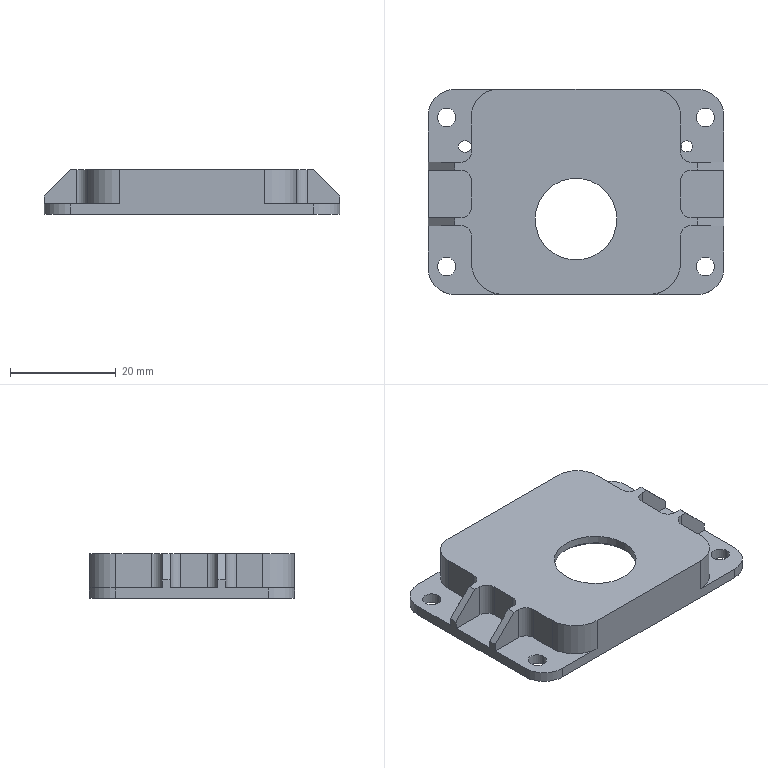NC program | NX | posted with a generic post | part box 56 x 38.85 x 8.5 mm
Lines 291 to 2522 of 3190, first 1751 of 2228 lines:
(CAVITY_MILL_COPY_COPY , TOOL : D4)
N556 T11 M6
N558 G54
N560 G17 G0 G90 X-11.864 Y14.625 S9500 M3
N562 G43 Z30. H11
N564 Z0.6
N566 G94 G1 Z-0.4 F1000.
N568 X-12.037 Y14.925
N570 G3 X-12.903 Y15.425 R1.
N572 G1 X-14.7 F1400.
N574 G3 X-15.8 Y14.325 R1.1
N576 G1 Y12.528
N578 G3 X-15.3 Y11.662 R1.
N580 G1 X-15. Y11.489
N582 Z0.6
N584 G0 Z30.
N586 X-11.764 Y14.525
N588 Z0.2
N590 G1 Z-0.8 F1000.
N592 X-11.937 Y14.825
N594 G3 X-12.803 Y15.325 R1.
N596 G1 X-14.7 F1400.
N598 G3 X-15.7 Y14.325 R1.
N600 G1 Y12.428
N602 G3 X-15.2 Y11.562 R1.
N604 G1 X-14.9 Y11.389
N606 Z0.2
N608 G0 X-11.764 Y14.525 Z-0.2
N610 G1 Z-1.2 F1000.
N612 X-11.937 Y14.825
N614 G3 X-12.803 Y15.325 R1.
N616 G1 X-14.7 F1400.
N618 G3 X-15.7 Y14.325 R1.
N620 G1 Y12.428
N622 G3 X-15.2 Y11.562 R1.
N624 G1 X-14.9 Y11.389
N626 Z-0.2
N628 G0 X-11.764 Y14.525 Z-0.6
N630 G1 Z-1.6 F1000.
N632 X-11.937 Y14.825
N634 G3 X-12.803 Y15.325 R1.
N636 G1 X-14.7 F1400.
N638 G3 X-15.7 Y14.325 R1.
N640 G1 Y12.428
N642 G3 X-15.2 Y11.562 R1.
N644 G1 X-14.9 Y11.389
N646 Z-0.6
N648 G0 X-11.764 Y14.525 Z-1.
N650 G1 Z-2. F1000.
N652 X-11.937 Y14.825
N654 G3 X-12.803 Y15.325 R1.
N656 G1 X-14.7 F1400.
N658 G3 X-15.7 Y14.325 R1.
N660 G1 Y12.428
N662 G3 X-15.2 Y11.562 R1.
N664 G1 X-14.9 Y11.389
N666 Z-1.
N668 G0 X-11.764 Y14.525 Z-1.375
N670 G1 Z-2.375 F1000.
N672 X-11.937 Y14.825
N674 G3 X-12.803 Y15.325 R1.
N676 G1 X-14.7 F1400.
N678 G3 X-15.7 Y14.325 R1.
N680 G1 Y12.428
N682 G3 X-15.2 Y11.562 R1.
N684 G1 X-14.9 Y11.389
N686 Z-1.375
N688 G0 X-11.764 Y14.525 Z-1.75
N690 G1 Z-2.75 F1000.
N692 X-11.937 Y14.825
N694 G3 X-12.803 Y15.325 R1.
N696 G1 X-14.7 F1400.
N698 G3 X-15.7 Y14.325 R1.
N700 G1 Y12.428
N702 G3 X-15.2 Y11.562 R1.
N704 G1 X-14.9 Y11.389
N706 Z-1.75
N708 G0 X-11.764 Y14.525 Z-2.125
N710 G1 Z-3.125 F1000.
N712 X-11.937 Y14.825
N714 G3 X-12.803 Y15.325 R1.
N716 G1 X-14.7 F1400.
N718 G3 X-15.7 Y14.325 R1.
N720 G1 Y12.428
N722 G3 X-15.2 Y11.562 R1.
N724 G1 X-14.9 Y11.389
N726 Z-2.125
N728 G0 X-11.764 Y14.525 Z-2.5
N730 G1 Z-3.5 F1000.
N732 X-11.937 Y14.825
N734 G3 X-12.803 Y15.325 R1.
N736 G1 X-14.7 F1400.
N738 G3 X-15.7 Y14.325 R1.
N740 G1 Y12.428
N742 G3 X-15.2 Y11.562 R1.
N744 G1 X-14.9 Y11.389
N746 Z-2.5
N748 G0 X-6.729 Y4.936 Z-2.875
N750 G1 Z-3.875 F1000.
N752 X-7.565 Y4.93
N754 G3 X-8.427 Y4.423 R1.
N756 G1 X-13.24 Y7.152
N758 G2 X-13.3 Y7.825 R3.8 F1400.
N760 G1 Y13.525
N762 X-13.9
N764 Y7.152
N766 X-13.24
N768 X-11.468 Y7.471
N770 G2 X-11.5 Y7.825 R2.
N772 G1 Y15.325
N774 X-14.7
N776 G3 X-15.7 Y14.325 R1.
N778 G1 Y5.352
N780 X-11.2
N782 G2 X-9.2 Y3.352 R2.
N784 G1 Y3.145
N786 G3 X-8.728 Y3.565 R0.5
N788 G2 X-7.411 Y5.416 R2.56
N790 G3 X-7.17 Y6.005 R0.5
N792 G2 X-8. Y5.825 R2.
N794 G1 X-9.5
N796 G2 X-11.468 Y7.471 R2.
N798 G3 X-11.579 Y7.705 R0.5
N800 G1 Z-2.875
N802 G0 X-6.729 Y4.936 Z-3.25
N804 G1 Z-4.25 F1000.
N806 X-7.565 Y4.93
N808 G3 X-8.427 Y4.423 R1.
N810 G1 X-13.24 Y7.152
N812 G2 X-13.3 Y7.825 R3.8 F1400.
N814 G1 Y13.525
N816 X-13.9
N818 Y7.152
N820 X-13.24
N822 X-11.468 Y7.471
N824 G2 X-11.5 Y7.825 R2.
N826 G1 Y15.325
N828 X-14.7
N830 G3 X-15.7 Y14.325 R1.
N832 G1 Y5.352
N834 X-11.2
N836 G2 X-9.2 Y3.352 R2.
N838 G1 Y3.145
N840 G3 X-8.728 Y3.565 R0.5
N842 G2 X-7.411 Y5.416 R2.56
N844 G3 X-7.17 Y6.005 R0.5
N846 G2 X-8. Y5.825 R2.
N848 G1 X-9.5
N850 G2 X-11.468 Y7.471 R2.
N852 G3 X-11.579 Y7.705 R0.5
N854 G1 Z-3.25
N856 G0 Z30.
N858 X-6.729 Y4.936
N860 Z-3.625
N862 G1 Z-4.625 F1000.
N864 X-7.565 Y4.93
N866 G3 X-8.427 Y4.423 R1.
N868 G1 X-13.24 Y7.152
N870 G2 X-13.3 Y7.825 R3.8 F1400.
N872 G1 Y13.525
N874 X-13.9
N876 Y7.152
N878 X-13.24
N880 X-11.468 Y7.471
N882 G2 X-11.5 Y7.825 R2.
N884 G1 Y15.325
N886 X-14.7
N888 G3 X-15.7 Y14.325 R1.
N890 G1 Y5.352
N892 X-11.2
N894 G2 X-9.2 Y3.352 R2.
N896 G1 Y3.145
N898 G3 X-8.728 Y3.565 R0.5
N900 G2 X-7.411 Y5.416 R2.56
N902 G3 X-7.17 Y6.005 R0.5
N904 G2 X-8. Y5.825 R2.
N906 G1 X-9.5
N908 G2 X-11.468 Y7.471 R2.
N910 G3 X-11.579 Y7.705 R0.5
N912 G1 Z-3.625
N914 G0 Z30.
N916 X-6.729 Y4.936
N918 Z-4.
N920 G1 Z-5. F1000.
N922 X-7.565 Y4.93
N924 G3 X-8.427 Y4.423 R1.
N926 G1 X-13.24 Y7.152
N928 G2 X-13.3 Y7.825 R3.8 F1400.
N930 G1 Y13.525
N932 X-13.9
N934 Y7.152
N936 X-13.24
N938 X-11.468 Y7.471
N940 G2 X-11.5 Y7.825 R2.
N942 G1 Y15.325
N944 X-14.7
N946 G3 X-15.7 Y14.325 R1.
N948 G1 Y5.352
N950 X-11.2
N952 G2 X-9.2 Y3.352 R2.
N954 G1 Y3.145
N956 G3 X-8.728 Y3.565 R0.5
N958 G2 X-7.411 Y5.416 R2.56
N960 G3 X-7.17 Y6.005 R0.5
N962 G2 X-8. Y5.825 R2.
N964 G1 X-9.5
N966 G2 X-11.468 Y7.471 R2.
N968 G3 X-11.579 Y7.705 R0.5
N970 G1 Z-4.
N972 G0 Z30.
N974 X-6.729 Y4.936
N976 Z-4.375
N978 G1 Z-5.375 F1000.
N980 X-7.565 Y4.93
N982 G3 X-8.427 Y4.423 R1.
N984 G1 X-13.24 Y7.152
N986 G2 X-13.3 Y7.825 R3.8 F1400.
N988 G1 Y13.525
N990 X-13.9
N992 Y7.152
N994 X-13.24
N996 X-11.468 Y7.471
N998 G2 X-11.5 Y7.825 R2.
N1000 G1 Y15.325
N1002 X-14.7
N1004 G3 X-15.7 Y14.325 R1.
N1006 G1 Y5.352
N1008 X-11.2
N1010 G2 X-9.2 Y3.352 R2.
N1012 G1 Y3.145
N1014 G3 X-8.728 Y3.565 R0.5
N1016 G2 X-7.411 Y5.416 R2.56
N1018 G3 X-7.17 Y6.005 R0.5
N1020 G2 X-8. Y5.825 R2.
N1022 G1 X-9.5
N1024 G2 X-11.468 Y7.471 R2.
N1026 G3 X-11.579 Y7.705 R0.5
N1028 G1 Z-4.375
N1030 G0 Z30.
N1032 X-6.729 Y4.936
N1034 Z-4.75
N1036 G1 Z-5.75 F1000.
N1038 X-7.565 Y4.93
N1040 G3 X-8.427 Y4.423 R1.
N1042 G1 X-13.24 Y7.152
N1044 G2 X-13.3 Y7.825 R3.8 F1400.
N1046 G1 Y13.525
N1048 X-13.9
N1050 Y7.152
N1052 X-13.24
N1054 X-11.468 Y7.471
N1056 G2 X-11.5 Y7.825 R2.
N1058 G1 Y15.325
N1060 X-14.7
N1062 G3 X-15.7 Y14.325 R1.
N1064 G1 Y5.352
N1066 X-11.2
N1068 G2 X-9.2 Y3.352 R2.
N1070 G1 Y3.145
N1072 G3 X-8.728 Y3.565 R0.5
N1074 G2 X-7.411 Y5.416 R2.56
N1076 G3 X-7.17 Y6.005 R0.5
N1078 G2 X-8. Y5.825 R2.
N1080 G1 X-9.5
N1082 G2 X-11.468 Y7.471 R2.
N1084 G3 X-11.579 Y7.705 R0.5
N1086 G1 Z-4.75
N1088 G0 Z30.
N1090 X-6.729 Y4.936
N1092 Z-5.125
N1094 G1 Z-6.125 F1000.
N1096 X-7.565 Y4.93
N1098 G3 X-8.427 Y4.423 R1.
N1100 G1 X-13.24 Y7.152
N1102 G2 X-13.3 Y7.825 R3.8 F1400.
N1104 G1 Y13.525
N1106 X-13.9
N1108 Y7.152
N1110 X-13.24
N1112 X-11.468 Y7.471
N1114 G2 X-11.5 Y7.825 R2.
N1116 G1 Y15.325
N1118 X-14.7
N1120 G3 X-15.7 Y14.325 R1.
N1122 G1 Y5.352
N1124 X-11.2
N1126 G2 X-9.2 Y3.352 R2.
N1128 G1 Y3.145
N1130 G3 X-8.728 Y3.565 R0.5
N1132 G2 X-7.411 Y5.416 R2.56
N1134 G3 X-7.17 Y6.005 R0.5
N1136 G2 X-8. Y5.825 R2.
N1138 G1 X-9.5
N1140 G2 X-11.468 Y7.471 R2.
N1142 G3 X-11.579 Y7.705 R0.5
N1144 G1 Z-5.125
N1146 G0 Z30.
N1148 X-6.729 Y4.936
N1150 Z-5.5
N1152 G1 Z-6.5 F1000.
N1154 X-7.565 Y4.93
N1156 G3 X-8.427 Y4.423 R1.
N1158 G1 X-13.24 Y7.152
N1160 G2 X-13.3 Y7.825 R3.8 F1400.
N1162 G1 Y13.525
N1164 X-13.9
N1166 Y7.152
N1168 X-13.24
N1170 X-11.468 Y7.471
N1172 G2 X-11.5 Y7.825 R2.
N1174 G1 Y15.325
N1176 X-14.7
N1178 G3 X-15.7 Y14.325 R1.
N1180 G1 Y5.352
N1182 X-11.2
N1184 G2 X-9.2 Y3.352 R2.
N1186 G1 Y3.145
N1188 G3 X-8.728 Y3.565 R0.5
N1190 G2 X-7.411 Y5.416 R2.56
N1192 G3 X-7.17 Y6.005 R0.5
N1194 G2 X-8. Y5.825 R2.
N1196 G1 X-9.5
N1198 G2 X-11.468 Y7.471 R2.
N1200 G3 X-11.579 Y7.705 R0.5
N1202 G1 Z-5.5
N1204 G0 Z30.
N1206 X-1.859 Y5.254
N1208 Z-2.875
N1210 G1 Z-3.875 F1000.
N1212 X-1.824 Y5.407
N1214 G3 X-2.115 Y6.363 R1.
N1216 G2 X-2.75 Y7.825 R2. F1400.
N1218 G1 Y15.325
N1220 X-6.
N1222 Y7.825
N1224 G2 X-6.635 Y6.363 R2.
N1226 G3 X-6.926 Y5.407 R1.
N1228 G1 X-6.891 Y5.254
N1230 Z-2.875
N1232 G0 X-1.859 Z-3.25
N1234 G1 Z-4.25 F1000.
N1236 X-1.824 Y5.407
N1238 G3 X-2.115 Y6.363 R1.
N1240 G2 X-2.75 Y7.825 R2. F1400.
N1242 G1 Y15.325
N1244 X-6.
N1246 Y7.825
N1248 G2 X-6.635 Y6.363 R2.
N1250 G3 X-6.926 Y5.407 R1.
N1252 G1 X-6.891 Y5.254
N1254 Z-3.25
N1256 G0 X-1.859 Z-3.625
N1258 G1 Z-4.625 F1000.
N1260 X-1.824 Y5.407
N1262 G3 X-2.115 Y6.363 R1.
N1264 G2 X-2.75 Y7.825 R2. F1400.
N1266 G1 Y15.325
N1268 X-6.
N1270 Y7.825
N1272 G2 X-6.635 Y6.363 R2.
N1274 G3 X-6.926 Y5.407 R1.
N1276 G1 X-6.891 Y5.254
N1278 Z-3.625
N1280 G0 X-1.859 Z-4.
N1282 G1 Z-5. F1000.
N1284 X-1.824 Y5.407
N1286 G3 X-2.115 Y6.363 R1.
N1288 G2 X-2.75 Y7.825 R2. F1400.
N1290 G1 Y15.325
N1292 X-6.
N1294 Y7.825
N1296 G2 X-6.635 Y6.363 R2.
N1298 G3 X-6.926 Y5.407 R1.
N1300 G1 X-6.891 Y5.254
N1302 Z-4.
N1304 G0 X-1.859 Z-4.375
N1306 G1 Z-5.375 F1000.
N1308 X-1.824 Y5.407
N1310 G3 X-2.115 Y6.363 R1.
N1312 G2 X-2.75 Y7.825 R2. F1400.
N1314 G1 Y15.325
N1316 X-6.
N1318 Y7.825
N1320 G2 X-6.635 Y6.363 R2.
N1322 G3 X-6.926 Y5.407 R1.
N1324 G1 X-6.891 Y5.254
N1326 Z-4.375
N1328 G0 X-1.859 Z-4.75
N1330 G1 Z-5.75 F1000.
N1332 X-1.824 Y5.407
N1334 G3 X-2.115 Y6.363 R1.
N1336 G2 X-2.75 Y7.825 R2. F1400.
N1338 G1 Y15.325
N1340 X-6.
N1342 Y7.825
N1344 G2 X-6.635 Y6.363 R2.
N1346 G3 X-6.926 Y5.407 R1.
N1348 G1 X-6.891 Y5.254
N1350 Z-4.75
N1352 G0 X-1.859 Z-5.125
N1354 G1 Z-6.125 F1000.
N1356 X-1.824 Y5.407
N1358 G3 X-2.115 Y6.363 R1.
N1360 G2 X-2.75 Y7.825 R2. F1400.
N1362 G1 Y15.325
N1364 X-6.
N1366 Y7.825
N1368 G2 X-6.635 Y6.363 R2.
N1370 G3 X-6.926 Y5.407 R1.
N1372 G1 X-6.891 Y5.254
N1374 Z-5.125
N1376 G0 X-1.859 Z-5.5
N1378 G1 Z-6.5 F1000.
N1380 X-1.824 Y5.407
N1382 G3 X-2.115 Y6.363 R1.
N1384 G2 X-2.75 Y7.825 R2. F1400.
N1386 G1 Y15.325
N1388 X-6.
N1390 Y7.825
N1392 G2 X-6.635 Y6.363 R2.
N1394 G3 X-6.926 Y5.407 R1.
N1396 G1 X-6.891 Y5.254
N1398 Z-5.5
N1400 G0 Z30.
N1402 X-8.502 Y1.101
N1404 Z-2.875
N1406 G1 Z-3.875 F1000.
N1408 X-8.659 Y1.116
N1410 G3 X-9.567 Y0.697 R1.
N1412 G2 X-11.2 Y-0.148 R2. F1400.
N1414 G1 X-15.7
N1416 Y-2.398
N1418 X-11.2
N1420 G2 X-9.567 Y-3.243 R2.
N1422 G3 X-8.659 Y-3.662 R1.
N1424 G1 X-8.502 Y-3.647
N1426 Z-2.875
N1428 G0 Y1.101 Z-3.25
N1430 G1 Z-4.25 F1000.
N1432 X-8.659 Y1.116
N1434 G3 X-9.567 Y0.697 R1.
N1436 G2 X-11.2 Y-0.148 R2. F1400.
N1438 G1 X-15.7
N1440 Y-2.398
N1442 X-11.2
N1444 G2 X-9.567 Y-3.243 R2.
N1446 G3 X-8.659 Y-3.662 R1.
N1448 G1 X-8.502 Y-3.647
N1450 Z-3.25
N1452 G0 Y1.101 Z-3.625
N1454 G1 Z-4.625 F1000.
N1456 X-8.659 Y1.116
N1458 G3 X-9.567 Y0.697 R1.
N1460 G2 X-11.2 Y-0.148 R2. F1400.
N1462 G1 X-15.7
N1464 Y-2.398
N1466 X-11.2
N1468 G2 X-9.567 Y-3.243 R2.
N1470 G3 X-8.659 Y-3.662 R1.
N1472 G1 X-8.502 Y-3.647
N1474 Z-3.625
N1476 G0 Y1.101 Z-4.
N1478 G1 Z-5. F1000.
N1480 X-8.659 Y1.116
N1482 G3 X-9.567 Y0.697 R1.
N1484 G2 X-11.2 Y-0.148 R2. F1400.
N1486 G1 X-15.7
N1488 Y-2.398
N1490 X-11.2
N1492 G2 X-9.567 Y-3.243 R2.
N1494 G3 X-8.659 Y-3.662 R1.
N1496 G1 X-8.502 Y-3.647
N1498 Z-4.
N1500 G0 Y1.101 Z-4.375
N1502 G1 Z-5.375 F1000.
N1504 X-8.659 Y1.116
N1506 G3 X-9.567 Y0.697 R1.
N1508 G2 X-11.2 Y-0.148 R2. F1400.
N1510 G1 X-15.7
N1512 Y-2.398
N1514 X-11.2
N1516 G2 X-9.567 Y-3.243 R2.
N1518 G3 X-8.659 Y-3.662 R1.
N1520 G1 X-8.502 Y-3.647
N1522 Z-4.375
N1524 G0 Y1.101 Z-4.75
N1526 G1 Z-5.75 F1000.
N1528 X-8.659 Y1.116
N1530 G3 X-9.567 Y0.697 R1.
N1532 G2 X-11.2 Y-0.148 R2. F1400.
N1534 G1 X-15.7
N1536 Y-2.398
N1538 X-11.2
N1540 G2 X-9.567 Y-3.243 R2.
N1542 G3 X-8.659 Y-3.662 R1.
N1544 G1 X-8.502 Y-3.647
N1546 Z-4.75
N1548 G0 Y1.101 Z-5.125
N1550 G1 Z-6.125 F1000.
N1552 X-8.659 Y1.116
N1554 G3 X-9.567 Y0.697 R1.
N1556 G2 X-11.2 Y-0.148 R2. F1400.
N1558 G1 X-15.7
N1560 Y-2.398
N1562 X-11.2
N1564 G2 X-9.567 Y-3.243 R2.
N1566 G3 X-8.659 Y-3.662 R1.
N1568 G1 X-8.502 Y-3.647
N1570 Z-5.125
N1572 G0 Y1.101 Z-5.5
N1574 G1 Z-6.5 F1000.
N1576 X-8.659 Y1.116
N1578 G3 X-9.567 Y0.697 R1.
N1580 G2 X-11.2 Y-0.148 R2. F1400.
N1582 G1 X-15.7
N1584 Y-2.398
N1586 X-11.2
N1588 G2 X-9.567 Y-3.243 R2.
N1590 G3 X-8.659 Y-3.662 R1.
N1592 G1 X-8.502 Y-3.647
N1594 Z-5.5
N1596 G0 Z30.
N1598 X-15. Y-11.489
N1600 Z0.6
N1602 G1 Z-0.4 F1000.
N1604 X-15.3 Y-11.662
N1606 G3 X-15.8 Y-12.528 R1.
N1608 G1 Y-14.325 F1400.
N1610 G3 X-14.7 Y-15.425 R1.1
N1612 G1 X-12.903
N1614 G3 X-12.037 Y-14.925 R1.
N1616 G1 X-11.864 Y-14.625
N1618 Z0.6
N1620 G0 Z30.
N1622 X-14.9 Y-11.389
N1624 Z0.2
N1626 G1 Z-0.8 F1000.
N1628 X-15.2 Y-11.562
N1630 G3 X-15.7 Y-12.428 R1.
N1632 G1 Y-14.325 F1400.
N1634 G3 X-14.7 Y-15.325 R1.
N1636 G1 X-12.803
N1638 G3 X-11.937 Y-14.825 R1.
N1640 G1 X-11.764 Y-14.525
N1642 Z0.2
N1644 G0 X-14.9 Y-11.389 Z-0.2
N1646 G1 Z-1.2 F1000.
N1648 X-15.2 Y-11.562
N1650 G3 X-15.7 Y-12.428 R1.
N1652 G1 Y-14.325 F1400.
N1654 G3 X-14.7 Y-15.325 R1.
N1656 G1 X-12.803
N1658 G3 X-11.937 Y-14.825 R1.
N1660 G1 X-11.764 Y-14.525
N1662 Z-0.2
N1664 G0 X-14.9 Y-11.389 Z-0.6
N1666 G1 Z-1.6 F1000.
N1668 X-15.2 Y-11.562
N1670 G3 X-15.7 Y-12.428 R1.
N1672 G1 Y-14.325 F1400.
N1674 G3 X-14.7 Y-15.325 R1.
N1676 G1 X-12.803
N1678 G3 X-11.937 Y-14.825 R1.
N1680 G1 X-11.764 Y-14.525
N1682 Z-0.6
N1684 G0 X-14.9 Y-11.389 Z-1.
N1686 G1 Z-2. F1000.
N1688 X-15.2 Y-11.562
N1690 G3 X-15.7 Y-12.428 R1.
N1692 G1 Y-14.325 F1400.
N1694 G3 X-14.7 Y-15.325 R1.
N1696 G1 X-12.803
N1698 G3 X-11.937 Y-14.825 R1.
N1700 G1 X-11.764 Y-14.525
N1702 Z-1.
N1704 G0 X-14.9 Y-11.389 Z-1.375
N1706 G1 Z-2.375 F1000.
N1708 X-15.2 Y-11.562
N1710 G3 X-15.7 Y-12.428 R1.
N1712 G1 Y-14.325 F1400.
N1714 G3 X-14.7 Y-15.325 R1.
N1716 G1 X-12.803
N1718 G3 X-11.937 Y-14.825 R1.
N1720 G1 X-11.764 Y-14.525
N1722 Z-1.375
N1724 G0 X-14.9 Y-11.389 Z-1.75
N1726 G1 Z-2.75 F1000.
N1728 X-15.2 Y-11.562
N1730 G3 X-15.7 Y-12.428 R1.
N1732 G1 Y-14.325 F1400.
N1734 G3 X-14.7 Y-15.325 R1.
N1736 G1 X-12.803
N1738 G3 X-11.937 Y-14.825 R1.
N1740 G1 X-11.764 Y-14.525
N1742 Z-1.75
N1744 G0 X-14.9 Y-11.389 Z-2.125
N1746 G1 Z-3.125 F1000.
N1748 X-15.2 Y-11.562
N1750 G3 X-15.7 Y-12.428 R1.
N1752 G1 Y-14.325 F1400.
N1754 G3 X-14.7 Y-15.325 R1.
N1756 G1 X-12.803
N1758 G3 X-11.937 Y-14.825 R1.
N1760 G1 X-11.764 Y-14.525
N1762 Z-2.125
N1764 G0 X-14.9 Y-11.389 Z-2.5
N1766 G1 Z-3.5 F1000.
N1768 X-15.2 Y-11.562
N1770 G3 X-15.7 Y-12.428 R1.
N1772 G1 Y-14.325 F1400.
N1774 G3 X-14.7 Y-15.325 R1.
N1776 G1 X-12.803
N1778 G3 X-11.937 Y-14.825 R1.
N1780 G1 X-11.764 Y-14.525
N1782 Z-2.5
N1784 G0 X-8.624 Y-7.799 Z-2.875
N1786 G1 Z-3.875 F1000.
N1788 X-9.404 Y-8.56
N1790 G3 X-9.675 Y-9.523 R1.
N1792 G1 X-12.715 Y-10.298
N1794 X-13.3 F1400.
N1796 Y-11.607
N1798 G2 X-12.131 Y-10.298 R4.4
N1800 G1 X-12.715
N1802 Y-7.898
N1804 X-15.7
N1806 Y-14.325
N1808 G3 X-14.7 Y-15.325 R1.
N1810 G1 X-11.5
N1812 Y-13.825
N1814 G2 X-9.5 Y-11.825 R2.
N1816 G1 X-8.
N1818 G2 X-7.563 Y-11.873 R2.
N1820 G3 X-7.919 Y-11.345 R0.5
N1822 G2 X-9.419 Y-7.625 R2.56
N1824 G3 X-9.529 Y-6.997 R0.5
N1826 G2 X-11.2 Y-7.898 R2.
N1828 G1 X-12.715
N1830 G3 X-13.581 Y-8.398 R1.
N1832 G1 Z-2.875
N1834 G0 X-8.624 Y-7.799 Z-3.25
N1836 G1 Z-4.25 F1000.
N1838 X-9.404 Y-8.56
N1840 G3 X-9.675 Y-9.523 R1.
N1842 G1 X-12.715 Y-10.298
N1844 X-13.3 F1400.
N1846 Y-11.607
N1848 G2 X-12.131 Y-10.298 R4.4
N1850 G1 X-12.715
N1852 Y-7.898
N1854 X-15.7
N1856 Y-14.325
N1858 G3 X-14.7 Y-15.325 R1.
N1860 G1 X-11.5
N1862 Y-13.825
N1864 G2 X-9.5 Y-11.825 R2.
N1866 G1 X-8.
N1868 G2 X-7.563 Y-11.873 R2.
N1870 G3 X-7.919 Y-11.345 R0.5
N1872 G2 X-9.419 Y-7.625 R2.56
N1874 G3 X-9.529 Y-6.997 R0.5
N1876 G2 X-11.2 Y-7.898 R2.
N1878 G1 X-12.715
N1880 G3 X-13.581 Y-8.398 R1.
N1882 G1 Z-3.25
N1884 G0 X-8.624 Y-7.799 Z-3.625
N1886 G1 Z-4.625 F1000.
N1888 X-9.404 Y-8.56
N1890 G3 X-9.675 Y-9.523 R1.
N1892 G1 X-12.715 Y-10.298
N1894 X-13.3 F1400.
N1896 Y-11.607
N1898 G2 X-12.131 Y-10.298 R4.4
N1900 G1 X-12.715
N1902 Y-7.898
N1904 X-15.7
N1906 Y-14.325
N1908 G3 X-14.7 Y-15.325 R1.
N1910 G1 X-11.5
N1912 Y-13.825
N1914 G2 X-9.5 Y-11.825 R2.
N1916 G1 X-8.
N1918 G2 X-7.563 Y-11.873 R2.
N1920 G3 X-7.919 Y-11.345 R0.5
N1922 G2 X-9.419 Y-7.625 R2.56
N1924 G3 X-9.529 Y-6.997 R0.5
N1926 G2 X-11.2 Y-7.898 R2.
N1928 G1 X-12.715
N1930 G3 X-13.581 Y-8.398 R1.
N1932 G1 Z-3.625
N1934 G0 X-8.624 Y-7.799 Z-4.
N1936 G1 Z-5. F1000.
N1938 X-9.404 Y-8.56
N1940 G3 X-9.675 Y-9.523 R1.
N1942 G1 X-12.715 Y-10.298
N1944 X-13.3 F1400.
N1946 Y-11.607
N1948 G2 X-12.131 Y-10.298 R4.4
N1950 G1 X-12.715
N1952 Y-7.898
N1954 X-15.7
N1956 Y-14.325
N1958 G3 X-14.7 Y-15.325 R1.
N1960 G1 X-11.5
N1962 Y-13.825
N1964 G2 X-9.5 Y-11.825 R2.
N1966 G1 X-8.
N1968 G2 X-7.563 Y-11.873 R2.
N1970 G3 X-7.919 Y-11.345 R0.5
N1972 G2 X-9.419 Y-7.625 R2.56
N1974 G3 X-9.529 Y-6.997 R0.5
N1976 G2 X-11.2 Y-7.898 R2.
N1978 G1 X-12.715
N1980 G3 X-13.581 Y-8.398 R1.
N1982 G1 Z-4.
N1984 G0 X-8.624 Y-7.799 Z-4.375
N1986 G1 Z-5.375 F1000.
N1988 X-9.404 Y-8.56
N1990 G3 X-9.675 Y-9.523 R1.
N1992 G1 X-12.715 Y-10.298
N1994 X-13.3 F1400.
N1996 Y-11.607
N1998 G2 X-12.131 Y-10.298 R4.4
N2000 G1 X-12.715
N2002 Y-7.898
N2004 X-15.7
N2006 Y-14.325
N2008 G3 X-14.7 Y-15.325 R1.
N2010 G1 X-11.5
N2012 Y-13.825
N2014 G2 X-9.5 Y-11.825 R2.
N2016 G1 X-8.
N2018 G2 X-7.563 Y-11.873 R2.
N2020 G3 X-7.919 Y-11.345 R0.5
N2022 G2 X-9.419 Y-7.625 R2.56
N2024 G3 X-9.529 Y-6.997 R0.5
N2026 G2 X-11.2 Y-7.898 R2.
N2028 G1 X-12.715
N2030 G3 X-13.581 Y-8.398 R1.
N2032 G1 Z-4.375
N2034 G0 X-8.624 Y-7.799 Z-4.75
N2036 G1 Z-5.75 F1000.
N2038 X-9.404 Y-8.56
N2040 G3 X-9.675 Y-9.523 R1.
N2042 G1 X-12.715 Y-10.298
N2044 X-13.3 F1400.
N2046 Y-11.607
N2048 G2 X-12.131 Y-10.298 R4.4
N2050 G1 X-12.715
N2052 Y-7.898
N2054 X-15.7
N2056 Y-14.325
N2058 G3 X-14.7 Y-15.325 R1.
N2060 G1 X-11.5
N2062 Y-13.825
N2064 G2 X-9.5 Y-11.825 R2.
N2066 G1 X-8.
N2068 G2 X-7.563 Y-11.873 R2.
N2070 G3 X-7.919 Y-11.345 R0.5
N2072 G2 X-9.419 Y-7.625 R2.56
N2074 G3 X-9.529 Y-6.997 R0.5
N2076 G2 X-11.2 Y-7.898 R2.
N2078 G1 X-12.715
N2080 G3 X-13.581 Y-8.398 R1.
N2082 G1 Z-4.75
N2084 G0 X-8.624 Y-7.799 Z-5.125
N2086 G1 Z-6.125 F1000.
N2088 X-9.404 Y-8.56
N2090 G3 X-9.675 Y-9.523 R1.
N2092 G1 X-12.715 Y-10.298
N2094 X-13.3 F1400.
N2096 Y-11.607
N2098 G2 X-12.131 Y-10.298 R4.4
N2100 G1 X-12.715
N2102 Y-7.898
N2104 X-15.7
N2106 Y-14.325
N2108 G3 X-14.7 Y-15.325 R1.
N2110 G1 X-11.5
N2112 Y-13.825
N2114 G2 X-9.5 Y-11.825 R2.
N2116 G1 X-8.
N2118 G2 X-7.563 Y-11.873 R2.
N2120 G3 X-7.919 Y-11.345 R0.5
N2122 G2 X-9.419 Y-7.625 R2.56
N2124 G3 X-9.529 Y-6.997 R0.5
N2126 G2 X-11.2 Y-7.898 R2.
N2128 G1 X-12.715
N2130 G3 X-13.581 Y-8.398 R1.
N2132 G1 Z-5.125
N2134 G0 X-8.624 Y-7.799 Z-5.5
N2136 G1 Z-6.5 F1000.
N2138 X-9.404 Y-8.56
N2140 G3 X-9.675 Y-9.523 R1.
N2142 G1 X-12.715 Y-10.298
N2144 X-13.3 F1400.
N2146 Y-11.607
N2148 G2 X-12.131 Y-10.298 R4.4
N2150 G1 X-12.715
N2152 Y-7.898
N2154 X-15.7
N2156 Y-14.325
N2158 G3 X-14.7 Y-15.325 R1.
N2160 G1 X-11.5
N2162 Y-13.825
N2164 G2 X-9.5 Y-11.825 R2.
N2166 G1 X-8.
N2168 G2 X-7.563 Y-11.873 R2.
N2170 G3 X-7.919 Y-11.345 R0.5
N2172 G2 X-9.419 Y-7.625 R2.56
N2174 G3 X-9.529 Y-6.997 R0.5
N2176 G2 X-11.2 Y-7.898 R2.
N2178 G1 X-12.715
N2180 G3 X-13.581 Y-8.398 R1.
N2182 G1 Z-5.5
N2184 G0 Z30.
N2186 X-5.874 Y-12.003
N2188 Z-2.875
N2190 G1 Z-3.875 F1000.
N2192 X-5.973 Y-12.125
N2194 G3 X-6.131 Y-13.112 R1.
N2196 G2 X-6. Y-13.825 R2. F1400.
N2198 G1 Y-15.325
N2200 X-3.333
N2202 G3 X-2.467 Y-14.825 R1.
N2204 G1 X-2.294 Y-14.525
N2206 Z-2.875
N2208 G0 X-5.874 Y-12.003 Z-3.25
N2210 G1 Z-4.25 F1000.
N2212 X-5.973 Y-12.125
N2214 G3 X-6.131 Y-13.112 R1.
N2216 G2 X-6. Y-13.825 R2. F1400.
N2218 G1 Y-15.325
N2220 X-3.333
N2222 G3 X-2.467 Y-14.825 R1.
N2224 G1 X-2.294 Y-14.525
N2226 Z-3.25
N2228 G0 X-5.874 Y-12.003 Z-3.625
N2230 G1 Z-4.625 F1000.
N2232 X-5.973 Y-12.125
N2234 G3 X-6.131 Y-13.112 R1.
N2236 G2 X-6. Y-13.825 R2. F1400.
N2238 G1 Y-15.325
N2240 X-3.333
N2242 G3 X-2.467 Y-14.825 R1.
N2244 G1 X-2.294 Y-14.525
N2246 Z-3.625
N2248 G0 X-5.874 Y-12.003 Z-4.
N2250 G1 Z-5. F1000.
N2252 X-5.973 Y-12.125
N2254 G3 X-6.131 Y-13.112 R1.
N2256 G2 X-6. Y-13.825 R2. F1400.
N2258 G1 Y-15.325
N2260 X-3.333
N2262 G3 X-2.467 Y-14.825 R1.
N2264 G1 X-2.294 Y-14.525
N2266 Z-4.
N2268 G0 X-5.874 Y-12.003 Z-4.375
N2270 G1 Z-5.375 F1000.
N2272 X-5.973 Y-12.125
N2274 G3 X-6.131 Y-13.112 R1.
N2276 G2 X-6. Y-13.825 R2. F1400.
N2278 G1 Y-15.325
N2280 X-3.333
N2282 G3 X-2.467 Y-14.825 R1.
N2284 G1 X-2.294 Y-14.525
N2286 Z-4.375
N2288 G0 X-5.874 Y-12.003 Z-4.75
N2290 G1 Z-5.75 F1000.
N2292 X-5.973 Y-12.125
N2294 G3 X-6.131 Y-13.112 R1.
N2296 G2 X-6. Y-13.825 R2. F1400.
N2298 G1 Y-15.325
N2300 X-3.333
N2302 G3 X-2.467 Y-14.825 R1.
N2304 G1 X-2.294 Y-14.525
N2306 Z-4.75
N2308 G0 X-5.874 Y-12.003 Z-5.125
N2310 G1 Z-6.125 F1000.
N2312 X-5.973 Y-12.125
N2314 G3 X-6.131 Y-13.112 R1.
N2316 G2 X-6. Y-13.825 R2. F1400.
N2318 G1 Y-15.325
N2320 X-3.333
N2322 G3 X-2.467 Y-14.825 R1.
N2324 G1 X-2.294 Y-14.525
N2326 Z-5.125
N2328 G0 X-5.874 Y-12.003 Z-5.5
N2330 G1 Z-6.5 F1000.
N2332 X-5.973 Y-12.125
N2334 G3 X-6.131 Y-13.112 R1.
N2336 G2 X-6. Y-13.825 R2. F1400.
N2338 G1 Y-15.325
N2340 X-3.333
N2342 G3 X-2.467 Y-14.825 R1.
N2344 G1 X-2.294 Y-14.525
N2346 Z-5.5
N2348 G0 Z30.
N2350 X2.294
N2352 Z-2.875
N2354 G1 Z-3.875 F1000.
N2356 X2.467 Y-14.825
N2358 G3 X3.333 Y-15.325 R1.
N2360 G1 X6. F1400.
N2362 Y-13.825
N2364 G2 X6.131 Y-13.112 R2.
N2366 G3 X5.973 Y-12.125 R1.
N2368 G1 X5.874 Y-12.003
N2370 Z-2.875
N2372 G0 X2.294 Y-14.525 Z-3.25
N2374 G1 Z-4.25 F1000.
N2376 X2.467 Y-14.825
N2378 G3 X3.333 Y-15.325 R1.
N2380 G1 X6. F1400.
N2382 Y-13.825
N2384 G2 X6.131 Y-13.112 R2.
N2386 G3 X5.973 Y-12.125 R1.
N2388 G1 X5.874 Y-12.003
N2390 Z-3.25
N2392 G0 X2.294 Y-14.525 Z-3.625
N2394 G1 Z-4.625 F1000.
N2396 X2.467 Y-14.825
N2398 G3 X3.333 Y-15.325 R1.
N2400 G1 X6. F1400.
N2402 Y-13.825
N2404 G2 X6.131 Y-13.112 R2.
N2406 G3 X5.973 Y-12.125 R1.
N2408 G1 X5.874 Y-12.003
N2410 Z-3.625
N2412 G0 X2.294 Y-14.525 Z-4.
N2414 G1 Z-5. F1000.
N2416 X2.467 Y-14.825
N2418 G3 X3.333 Y-15.325 R1.
N2420 G1 X6. F1400.
N2422 Y-13.825
N2424 G2 X6.131 Y-13.112 R2.
N2426 G3 X5.973 Y-12.125 R1.
N2428 G1 X5.874 Y-12.003
N2430 Z-4.
N2432 G0 X2.294 Y-14.525 Z-4.375
N2434 G1 Z-5.375 F1000.
N2436 X2.467 Y-14.825
N2438 G3 X3.333 Y-15.325 R1.
N2440 G1 X6. F1400.
N2442 Y-13.825
N2444 G2 X6.131 Y-13.112 R2.
N2446 G3 X5.973 Y-12.125 R1.
N2448 G1 X5.874 Y-12.003
N2450 Z-4.375
N2452 G0 X2.294 Y-14.525 Z-4.75
N2454 G1 Z-5.75 F1000.
N2456 X2.467 Y-14.825
N2458 G3 X3.333 Y-15.325 R1.
N2460 G1 X6. F1400.
N2462 Y-13.825
N2464 G2 X6.131 Y-13.112 R2.
N2466 G3 X5.973 Y-12.125 R1.
N2468 G1 X5.874 Y-12.003
N2470 Z-4.75
N2472 G0 X2.294 Y-14.525 Z-5.125
N2474 G1 Z-6.125 F1000.
N2476 X2.467 Y-14.825
N2478 G3 X3.333 Y-15.325 R1.
N2480 G1 X6. F1400.
N2482 Y-13.825
N2484 G2 X6.131 Y-13.112 R2.
N2486 G3 X5.973 Y-12.125 R1.
N2488 G1 X5.874 Y-12.003
N2490 Z-5.125
N2492 G0 X2.294 Y-14.525 Z-5.5
N2494 G1 Z-6.5 F1000.
N2496 X2.467 Y-14.825
N2498 G3 X3.333 Y-15.325 R1.
N2500 G1 X6. F1400.
N2502 Y-13.825
N2504 G2 X6.131 Y-13.112 R2.
N2506 G3 X5.973 Y-12.125 R1.
N2508 G1 X5.874 Y-12.003
N2510 Z-5.5
N2512 G0 Z30.
N2514 X11.864 Y-14.625
N2516 Z0.6
N2518 G1 Z-0.4 F1000.
N2520 X12.037 Y-14.925
N2522 G3 X12.903 Y-15.425 R1.
N2524 G1 X14.7 F1400.
N2526 G3 X15.8 Y-14.325 R1.1
N2528 G1 Y-12.528
N2530 G3 X15.3 Y-11.662 R1.
N2532 G1 X15. Y-11.489
N2534 Z0.6
N2536 G0 Z30.
N2538 X11.764 Y-14.525
N2540 Z0.2
N2542 G1 Z-0.8 F1000.
N2544 X11.937 Y-14.825
N2546 G3 X12.803 Y-15.325 R1.
N2548 G1 X14.7 F1400.
N2550 G3 X15.7 Y-14.325 R1.
N2552 G1 Y-12.428
N2554 G3 X15.2 Y-11.562 R1.
N2556 G1 X14.9 Y-11.389
N2558 Z0.2
N2560 G0 X11.764 Y-14.525 Z-0.2
N2562 G1 Z-1.2 F1000.
N2564 X11.937 Y-14.825
N2566 G3 X12.803 Y-15.325 R1.
N2568 G1 X14.7 F1400.
N2570 G3 X15.7 Y-14.325 R1.
N2572 G1 Y-12.428
N2574 G3 X15.2 Y-11.562 R1.
N2576 G1 X14.9 Y-11.389
N2578 Z-0.2
N2580 G0 X11.764 Y-14.525 Z-0.6
N2582 G1 Z-1.6 F1000.
N2584 X11.937 Y-14.825
N2586 G3 X12.803 Y-15.325 R1.
N2588 G1 X14.7 F1400.
N2590 G3 X15.7 Y-14.325 R1.
N2592 G1 Y-12.428
N2594 G3 X15.2 Y-11.562 R1.
N2596 G1 X14.9 Y-11.389
N2598 Z-0.6
N2600 G0 X11.764 Y-14.525 Z-1.
N2602 G1 Z-2. F1000.
N2604 X11.937 Y-14.825
N2606 G3 X12.803 Y-15.325 R1.
N2608 G1 X14.7 F1400.
N2610 G3 X15.7 Y-14.325 R1.
N2612 G1 Y-12.428
N2614 G3 X15.2 Y-11.562 R1.
N2616 G1 X14.9 Y-11.389
N2618 Z-1.
N2620 G0 X11.764 Y-14.525 Z-1.375
N2622 G1 Z-2.375 F1000.
N2624 X11.937 Y-14.825
N2626 G3 X12.803 Y-15.325 R1.
N2628 G1 X14.7 F1400.
N2630 G3 X15.7 Y-14.325 R1.
N2632 G1 Y-12.428
N2634 G3 X15.2 Y-11.562 R1.
N2636 G1 X14.9 Y-11.389
N2638 Z-1.375
N2640 G0 X11.764 Y-14.525 Z-1.75
N2642 G1 Z-2.75 F1000.
N2644 X11.937 Y-14.825
N2646 G3 X12.803 Y-15.325 R1.
N2648 G1 X14.7 F1400.
N2650 G3 X15.7 Y-14.325 R1.
N2652 G1 Y-12.428
N2654 G3 X15.2 Y-11.562 R1.
N2656 G1 X14.9 Y-11.389
N2658 Z-1.75
N2660 G0 X11.764 Y-14.525 Z-2.125
N2662 G1 Z-3.125 F1000.
N2664 X11.937 Y-14.825
N2666 G3 X12.803 Y-15.325 R1.
N2668 G1 X14.7 F1400.
N2670 G3 X15.7 Y-14.325 R1.
N2672 G1 Y-12.428
N2674 G3 X15.2 Y-11.562 R1.
N2676 G1 X14.9 Y-11.389
N2678 Z-2.125
N2680 G0 X11.764 Y-14.525 Z-2.5
N2682 G1 Z-3.5 F1000.
N2684 X11.937 Y-14.825
N2686 G3 X12.803 Y-15.325 R1.
N2688 G1 X14.7 F1400.
N2690 G3 X15.7 Y-14.325 R1.
N2692 G1 Y-12.428
N2694 G3 X15.2 Y-11.562 R1.
N2696 G1 X14.9 Y-11.389
N2698 Z-2.5
N2700 G0 X7.53 Y-10.639 Z-2.875
N2702 G1 Z-3.875 F1000.
N2704 X8.841 Y-10.401
N2706 G3 X9.604 Y-9.754 R1.
N2708 G1 X12.781 Y-10.894
N2710 G2 X13.3 Y-11.607 R4.4 F1400.
N2712 G1 Y-10.298
N2714 X12.131
N2716 G2 X12.781 Y-10.894 R4.4
N2718 G1 X10.991 Y-12.493
N2720 G2 X11.5 Y-13.825 R2.
N2722 G1 Y-15.325
N2724 X14.7
N2726 G3 X15.7 Y-14.325 R1.
N2728 G1 Y-7.898
N2730 X11.2
N2732 G2 X9.529 Y-6.997 R2.
N2734 G3 X9.419 Y-7.625 R0.5
N2736 G2 X7.919 Y-11.345 R2.56
N2738 G3 X7.563 Y-11.873 R0.5
N2740 G2 X8. Y-11.825 R2.
N2742 G1 X9.5
N2744 G2 X10.991 Y-12.493 R2.
N2746 G3 X11.941 Y-12.805 R1.
N2748 G1 Z-2.875
N2750 G0 X7.53 Y-10.639 Z-3.25
N2752 G1 Z-4.25 F1000.
N2754 X8.841 Y-10.401
N2756 G3 X9.604 Y-9.754 R1.
N2758 G1 X12.781 Y-10.894
N2760 G2 X13.3 Y-11.607 R4.4 F1400.
N2762 G1 Y-10.298
N2764 X12.131
N2766 G2 X12.781 Y-10.894 R4.4
N2768 G1 X10.991 Y-12.493
N2770 G2 X11.5 Y-13.825 R2.
N2772 G1 Y-15.325
N2774 X14.7
N2776 G3 X15.7 Y-14.325 R1.
N2778 G1 Y-7.898
N2780 X11.2
N2782 G2 X9.529 Y-6.997 R2.
N2784 G3 X9.419 Y-7.625 R0.5
N2786 G2 X7.919 Y-11.345 R2.56
N2788 G3 X7.563 Y-11.873 R0.5
N2790 G2 X8. Y-11.825 R2.
N2792 G1 X9.5
N2794 G2 X10.991 Y-12.493 R2.
N2796 G3 X11.941 Y-12.805 R1.
N2798 G1 Z-3.25
N2800 G0 X7.53 Y-10.639 Z-3.625
N2802 G1 Z-4.625 F1000.
N2804 X8.841 Y-10.401
N2806 G3 X9.604 Y-9.754 R1.
N2808 G1 X12.781 Y-10.894
N2810 G2 X13.3 Y-11.607 R4.4 F1400.
N2812 G1 Y-10.298
N2814 X12.131
N2816 G2 X12.781 Y-10.894 R4.4
N2818 G1 X10.991 Y-12.493
N2820 G2 X11.5 Y-13.825 R2.
N2822 G1 Y-15.325
N2824 X14.7
N2826 G3 X15.7 Y-14.325 R1.
N2828 G1 Y-7.898
N2830 X11.2
N2832 G2 X9.529 Y-6.997 R2.
N2834 G3 X9.419 Y-7.625 R0.5
N2836 G2 X7.919 Y-11.345 R2.56
N2838 G3 X7.563 Y-11.873 R0.5
N2840 G2 X8. Y-11.825 R2.
N2842 G1 X9.5
N2844 G2 X10.991 Y-12.493 R2.
N2846 G3 X11.941 Y-12.805 R1.
N2848 G1 Z-3.625
N2850 G0 X7.53 Y-10.639 Z-4.
N2852 G1 Z-5. F1000.
N2854 X8.841 Y-10.401
N2856 G3 X9.604 Y-9.754 R1.
N2858 G1 X12.781 Y-10.894
N2860 G2 X13.3 Y-11.607 R4.4 F1400.
N2862 G1 Y-10.298
N2864 X12.131
N2866 G2 X12.781 Y-10.894 R4.4
N2868 G1 X10.991 Y-12.493
N2870 G2 X11.5 Y-13.825 R2.
N2872 G1 Y-15.325
N2874 X14.7
N2876 G3 X15.7 Y-14.325 R1.
N2878 G1 Y-7.898
N2880 X11.2
N2882 G2 X9.529 Y-6.997 R2.
N2884 G3 X9.419 Y-7.625 R0.5
N2886 G2 X7.919 Y-11.345 R2.56
N2888 G3 X7.563 Y-11.873 R0.5
N2890 G2 X8. Y-11.825 R2.
N2892 G1 X9.5
N2894 G2 X10.991 Y-12.493 R2.
N2896 G3 X11.941 Y-12.805 R1.
N2898 G1 Z-4.
N2900 G0 X7.53 Y-10.639 Z-4.375
N2902 G1 Z-5.375 F1000.
N2904 X8.841 Y-10.401
N2906 G3 X9.604 Y-9.754 R1.
N2908 G1 X12.781 Y-10.894
N2910 G2 X13.3 Y-11.607 R4.4 F1400.
N2912 G1 Y-10.298
N2914 X12.131
N2916 G2 X12.781 Y-10.894 R4.4
N2918 G1 X10.991 Y-12.493
N2920 G2 X11.5 Y-13.825 R2.
N2922 G1 Y-15.325
N2924 X14.7
N2926 G3 X15.7 Y-14.325 R1.
N2928 G1 Y-7.898
N2930 X11.2
N2932 G2 X9.529 Y-6.997 R2.
N2934 G3 X9.419 Y-7.625 R0.5
N2936 G2 X7.919 Y-11.345 R2.56
N2938 G3 X7.563 Y-11.873 R0.5
N2940 G2 X8. Y-11.825 R2.
N2942 G1 X9.5
N2944 G2 X10.991 Y-12.493 R2.
N2946 G3 X11.941 Y-12.805 R1.
N2948 G1 Z-4.375
N2950 G0 X7.53 Y-10.639 Z-4.75
N2952 G1 Z-5.75 F1000.
N2954 X8.841 Y-10.401
N2956 G3 X9.604 Y-9.754 R1.
N2958 G1 X12.781 Y-10.894
N2960 G2 X13.3 Y-11.607 R4.4 F1400.
N2962 G1 Y-10.298
N2964 X12.131
N2966 G2 X12.781 Y-10.894 R4.4
N2968 G1 X10.991 Y-12.493
N2970 G2 X11.5 Y-13.825 R2.
N2972 G1 Y-15.325
N2974 X14.7
N2976 G3 X15.7 Y-14.325 R1.
N2978 G1 Y-7.898
N2980 X11.2
N2982 G2 X9.529 Y-6.997 R2.
N2984 G3 X9.419 Y-7.625 R0.5
N2986 G2 X7.919 Y-11.345 R2.56
N2988 G3 X7.563 Y-11.873 R0.5
N2990 G2 X8. Y-11.825 R2.
N2992 G1 X9.5
N2994 G2 X10.991 Y-12.493 R2.
N2996 G3 X11.941 Y-12.805 R1.
N2998 G1 Z-4.75
N3000 G0 X7.53 Y-10.639 Z-5.125
N3002 G1 Z-6.125 F1000.
N3004 X8.841 Y-10.401
N3006 G3 X9.604 Y-9.754 R1.
N3008 G1 X12.781 Y-10.894
N3010 G2 X13.3 Y-11.607 R4.4 F1400.
N3012 G1 Y-10.298
N3014 X12.131
N3016 G2 X12.781 Y-10.894 R4.4
N3018 G1 X10.991 Y-12.493
N3020 G2 X11.5 Y-13.825 R2.
N3022 G1 Y-15.325
N3024 X14.7
N3026 G3 X15.7 Y-14.325 R1.
N3028 G1 Y-7.898
N3030 X11.2
N3032 G2 X9.529 Y-6.997 R2.
N3034 G3 X9.419 Y-7.625 R0.5
N3036 G2 X7.919 Y-11.345 R2.56
N3038 G3 X7.563 Y-11.873 R0.5
N3040 G2 X8. Y-11.825 R2.
N3042 G1 X9.5
N3044 G2 X10.991 Y-12.493 R2.
N3046 G3 X11.941 Y-12.805 R1.
N3048 G1 Z-5.125
N3050 G0 X7.53 Y-10.639 Z-5.5
N3052 G1 Z-6.5 F1000.
N3054 X8.841 Y-10.401
N3056 G3 X9.604 Y-9.754 R1.
N3058 G1 X12.781 Y-10.894
N3060 G2 X13.3 Y-11.607 R4.4 F1400.
N3062 G1 Y-10.298
N3064 X12.131
N3066 G2 X12.781 Y-10.894 R4.4
N3068 G1 X10.991 Y-12.493
N3070 G2 X11.5 Y-13.825 R2.
N3072 G1 Y-15.325
N3074 X14.7
N3076 G3 X15.7 Y-14.325 R1.
N3078 G1 Y-7.898
N3080 X11.2
N3082 G2 X9.529 Y-6.997 R2.
N3084 G3 X9.419 Y-7.625 R0.5
N3086 G2 X7.919 Y-11.345 R2.56
N3088 G3 X7.563 Y-11.873 R0.5
N3090 G2 X8. Y-11.825 R2.
N3092 G1 X9.5
N3094 G2 X10.991 Y-12.493 R2.
N3096 G3 X11.941 Y-12.805 R1.
N3098 G1 Z-5.5
N3100 G0 Z30.
N3102 X8.502 Y-3.647
N3104 Z-2.875
N3106 G1 Z-3.875 F1000.
N3108 X8.659 Y-3.662
N3110 G3 X9.567 Y-3.243 R1.
N3112 G2 X11.2 Y-2.398 R2. F1400.
N3114 G1 X15.7
N3116 Y-0.148
N3118 X11.2
N3120 G2 X9.567 Y0.697 R2.
N3122 G3 X8.659 Y1.116 R1.
N3124 G1 X8.502 Y1.101
N3126 Z-2.875
N3128 G0 Y-3.647 Z-3.25
N3130 G1 Z-4.25 F1000.
N3132 X8.659 Y-3.662
N3134 G3 X9.567 Y-3.243 R1.
N3136 G2 X11.2 Y-2.398 R2. F1400.
N3138 G1 X15.7
N3140 Y-0.148
N3142 X11.2
N3144 G2 X9.567 Y0.697 R2.
N3146 G3 X8.659 Y1.116 R1.
N3148 G1 X8.502 Y1.101
N3150 Z-3.25
N3152 G0 Y-3.647 Z-3.625
N3154 G1 Z-4.625 F1000.
N3156 X8.659 Y-3.662
N3158 G3 X9.567 Y-3.243 R1.
N3160 G2 X11.2 Y-2.398 R2. F1400.
N3162 G1 X15.7
N3164 Y-0.148
N3166 X11.2
N3168 G2 X9.567 Y0.697 R2.
N3170 G3 X8.659 Y1.116 R1.
N3172 G1 X8.502 Y1.101
N3174 Z-3.625
N3176 G0 Y-3.647 Z-4.
N3178 G1 Z-5. F1000.
N3180 X8.659 Y-3.662
N3182 G3 X9.567 Y-3.243 R1.
N3184 G2 X11.2 Y-2.398 R2. F1400.
N3186 G1 X15.7
N3188 Y-0.148
N3190 X11.2
N3192 G2 X9.567 Y0.697 R2.
N3194 G3 X8.659 Y1.116 R1.
N3196 G1 X8.502 Y1.101
N3198 Z-4.
N3200 G0 Y-3.647 Z-4.375
N3202 G1 Z-5.375 F1000.
N3204 X8.659 Y-3.662
N3206 G3 X9.567 Y-3.243 R1.
N3208 G2 X11.2 Y-2.398 R2. F1400.
N3210 G1 X15.7
N3212 Y-0.148
N3214 X11.2
N3216 G2 X9.567 Y0.697 R2.
N3218 G3 X8.659 Y1.116 R1.
N3220 G1 X8.502 Y1.101
N3222 Z-4.375
N3224 G0 Y-3.647 Z-4.75
N3226 G1 Z-5.75 F1000.
N3228 X8.659 Y-3.662
N3230 G3 X9.567 Y-3.243 R1.
N3232 G2 X11.2 Y-2.398 R2. F1400.
N3234 G1 X15.7
N3236 Y-0.148
N3238 X11.2
N3240 G2 X9.567 Y0.697 R2.
N3242 G3 X8.659 Y1.116 R1.
N3244 G1 X8.502 Y1.101
N3246 Z-4.75
N3248 G0 Y-3.647 Z-5.125
N3250 G1 Z-6.125 F1000.
N3252 X8.659 Y-3.662
N3254 G3 X9.567 Y-3.243 R1.
N3256 G2 X11.2 Y-2.398 R2. F1400.
N3258 G1 X15.7
N3260 Y-0.148
N3262 X11.2
N3264 G2 X9.567 Y0.697 R2.
N3266 G3 X8.659 Y1.116 R1.
N3268 G1 X8.502 Y1.101
N3270 Z-5.125
N3272 G0 Y-3.647 Z-5.5
N3274 G1 Z-6.5 F1000.
N3276 X8.659 Y-3.662
N3278 G3 X9.567 Y-3.243 R1.
N3280 G2 X11.2 Y-2.398 R2. F1400.
N3282 G1 X15.7
N3284 Y-0.148
N3286 X11.2
N3288 G2 X9.567 Y0.697 R2.
N3290 G3 X8.659 Y1.116 R1.
N3292 G1 X8.502 Y1.101
N3294 Z-5.5
N3296 G0 Z30.
N3298 X6.891 Y5.254
N3300 Z-2.875
N3302 G1 Z-3.875 F1000.
N3304 X6.926 Y5.407
N3306 G3 X6.635 Y6.363 R1.
N3308 G2 X6. Y7.825 R2. F1400.
N3310 G1 Y15.325
N3312 X2.75
N3314 Y7.825
N3316 G2 X2.115 Y6.363 R2.
N3318 G3 X1.824 Y5.407 R1.
N3320 G1 X1.859 Y5.254
N3322 Z-2.875
N3324 G0 X6.891 Z-3.25
N3326 G1 Z-4.25 F1000.
N3328 X6.926 Y5.407
N3330 G3 X6.635 Y6.363 R1.
N3332 G2 X6. Y7.825 R2. F1400.
N3334 G1 Y15.325
N3336 X2.75
N3338 Y7.825
N3340 G2 X2.115 Y6.363 R2.
N3342 G3 X1.824 Y5.407 R1.
N3344 G1 X1.859 Y5.254
N3346 Z-3.25
N3348 G0 X6.891 Z-3.625
N3350 G1 Z-4.625 F1000.
N3352 X6.926 Y5.407
N3354 G3 X6.635 Y6.363 R1.
N3356 G2 X6. Y7.825 R2. F1400.
N3358 G1 Y15.325
N3360 X2.75
N3362 Y7.825
N3364 G2 X2.115 Y6.363 R2.
N3366 G3 X1.824 Y5.407 R1.
N3368 G1 X1.859 Y5.254
N3370 Z-3.625
N3372 G0 X6.891 Z-4.
N3374 G1 Z-5. F1000.
N3376 X6.926 Y5.407
N3378 G3 X6.635 Y6.363 R1.
N3380 G2 X6. Y7.825 R2. F1400.
N3382 G1 Y15.325
N3384 X2.75
N3386 Y7.825
N3388 G2 X2.115 Y6.363 R2.
N3390 G3 X1.824 Y5.407 R1.
N3392 G1 X1.859 Y5.254
N3394 Z-4.
N3396 G0 X6.891 Z-4.375
N3398 G1 Z-5.375 F1000.
N3400 X6.926 Y5.407
N3402 G3 X6.635 Y6.363 R1.
N3404 G2 X6. Y7.825 R2. F1400.
N3406 G1 Y15.325
N3408 X2.75
N3410 Y7.825
N3412 G2 X2.115 Y6.363 R2.
N3414 G3 X1.824 Y5.407 R1.
N3416 G1 X1.859 Y5.254
N3418 Z-4.375
N3420 G0 X6.891 Z-4.75
N3422 G1 Z-5.75 F1000.
N3424 X6.926 Y5.407
N3426 G3 X6.635 Y6.363 R1.
N3428 G2 X6. Y7.825 R2. F1400.
N3430 G1 Y15.325
N3432 X2.75
N3434 Y7.825
N3436 G2 X2.115 Y6.363 R2.
N3438 G3 X1.824 Y5.407 R1.
N3440 G1 X1.859 Y5.254
N3442 Z-4.75
N3444 G0 X6.891 Z-5.125
N3446 G1 Z-6.125 F1000.
N3448 X6.926 Y5.407
N3450 G3 X6.635 Y6.363 R1.
N3452 G2 X6. Y7.825 R2. F1400.
N3454 G1 Y15.325
N3456 X2.75
N3458 Y7.825
N3460 G2 X2.115 Y6.363 R2.
N3462 G3 X1.824 Y5.407 R1.
N3464 G1 X1.859 Y5.254
N3466 Z-5.125
N3468 G0 X6.891 Z-5.5
N3470 G1 Z-6.5 F1000.
N3472 X6.926 Y5.407
N3474 G3 X6.635 Y6.363 R1.
N3476 G2 X6. Y7.825 R2. F1400.
N3478 G1 Y15.325
N3480 X2.75
N3482 Y7.825
N3484 G2 X2.115 Y6.363 R2.
N3486 G3 X1.824 Y5.407 R1.
N3488 G1 X1.859 Y5.254
N3490 Z-5.5
N3492 G0 Z30.
N3494 X15. Y11.489
N3496 Z0.6
N3498 G1 Z-0.4 F1000.
N3500 X15.3 Y11.662
N3502 G3 X15.8 Y12.528 R1.
N3504 G1 Y14.325 F1400.
N3506 G3 X14.7 Y15.425 R1.1
N3508 G1 X12.903
N3510 G3 X12.037 Y14.925 R1.
N3512 G1 X11.864 Y14.625
N3514 Z0.6
N3516 G0 Z30.
N3518 X14.9 Y11.389
N3520 Z0.2
N3522 G1 Z-0.8 F1000.
N3524 X15.2 Y11.562
N3526 G3 X15.7 Y12.428 R1.
N3528 G1 Y14.325 F1400.
N3530 G3 X14.7 Y15.325 R1.
N3532 G1 X12.803
N3534 G3 X11.937 Y14.825 R1.
N3536 G1 X11.764 Y14.525
N3538 Z0.2
N3540 G0 X14.9 Y11.389 Z-0.2
N3542 G1 Z-1.2 F1000.
N3544 X15.2 Y11.562
N3546 G3 X15.7 Y12.428 R1.
N3548 G1 Y14.325 F1400.
N3550 G3 X14.7 Y15.325 R1.
N3552 G1 X12.803
N3554 G3 X11.937 Y14.825 R1.
N3556 G1 X11.764 Y14.525
N3558 Z-0.2
N3560 G0 X14.9 Y11.389 Z-0.6
N3562 G1 Z-1.6 F1000.
N3564 X15.2 Y11.562
N3566 G3 X15.7 Y12.428 R1.
N3568 G1 Y14.325 F1400.
N3570 G3 X14.7 Y15.325 R1.
N3572 G1 X12.803
N3574 G3 X11.937 Y14.825 R1.
N3576 G1 X11.764 Y14.525
N3578 Z-0.6
N3580 G0 X14.9 Y11.389 Z-1.
N3582 G1 Z-2. F1000.
N3584 X15.2 Y11.562
N3586 G3 X15.7 Y12.428 R1.
N3588 G1 Y14.325 F1400.
N3590 G3 X14.7 Y15.325 R1.
N3592 G1 X12.803
N3594 G3 X11.937 Y14.825 R1.
N3596 G1 X11.764 Y14.525
N3598 Z-1.
N3600 G0 X14.9 Y11.389 Z-1.375
N3602 G1 Z-2.375 F1000.
N3604 X15.2 Y11.562
N3606 G3 X15.7 Y12.428 R1.
N3608 G1 Y14.325 F1400.
N3610 G3 X14.7 Y15.325 R1.
N3612 G1 X12.803
N3614 G3 X11.937 Y14.825 R1.
N3616 G1 X11.764 Y14.525
N3618 Z-1.375
N3620 G0 X14.9 Y11.389 Z-1.75
N3622 G1 Z-2.75 F1000.
N3624 X15.2 Y11.562
N3626 G3 X15.7 Y12.428 R1.
N3628 G1 Y14.325 F1400.
N3630 G3 X14.7 Y15.325 R1.
N3632 G1 X12.803
N3634 G3 X11.937 Y14.825 R1.
N3636 G1 X11.764 Y14.525
N3638 Z-1.75
N3640 G0 X14.9 Y11.389 Z-2.125
N3642 G1 Z-3.125 F1000.
N3644 X15.2 Y11.562
N3646 G3 X15.7 Y12.428 R1.
N3648 G1 Y14.325 F1400.
N3650 G3 X14.7 Y15.325 R1.
N3652 G1 X12.803
N3654 G3 X11.937 Y14.825 R1.
N3656 G1 X11.764 Y14.525
N3658 Z-2.125
N3660 G0 X14.9 Y11.389 Z-2.5
N3662 G1 Z-3.5 F1000.
N3664 X15.2 Y11.562
N3666 G3 X15.7 Y12.428 R1.
N3668 G1 Y14.325 F1400.
N3670 G3 X14.7 Y15.325 R1.
N3672 G1 X12.803
N3674 G3 X11.937 Y14.825 R1.
N3676 G1 X11.764 Y14.525
N3678 Z-2.5
N3680 G0 X8.142 Y2.92 Z-2.875
N3682 G1 Z-3.875 F1000.
N3684 X8.424 Y3.38
N3686 G3 X8.451 Y4.379 R1.
N3688 G1 X13.57 Y7.152
N3690 X13.9 F1400.
N3692 Y13.525
N3694 X13.3
N3696 Y7.825
N3698 G2 X13.24 Y7.152 R3.8
N3700 G1 X13.57
N3702 Y5.352
N3704 X15.7
N3706 Y14.325
N3708 G3 X14.7 Y15.325 R1.
N3710 G1 X11.5
N3712 Y7.825
N3714 G2 X9.5 Y5.825 R2.
N3716 G1 X8.
N3718 G2 X7.17 Y6.005 R2.
N3720 G3 X7.411 Y5.416 R0.5
N3722 G2 X8.728 Y3.565 R2.56
N3724 G3 X9.2 Y3.145 R0.5
N3726 G1 Y3.352
N3728 G2 X11.2 Y5.352 R2.
N3730 G1 X13.57
N3732 G3 X14.436 Y5.852 R1.
N3734 G1 Z-2.875
N3736 G0 X8.142 Y2.92 Z-3.25
N3738 G1 Z-4.25 F1000.
N3740 X8.424 Y3.38
N3742 G3 X8.451 Y4.379 R1.
N3744 G1 X13.57 Y7.152
N3746 X13.9 F1400.
N3748 Y13.525
N3750 X13.3
N3752 Y7.825
N3754 G2 X13.24 Y7.152 R3.8
N3756 G1 X13.57
N3758 Y5.352
N3760 X15.7
N3762 Y14.325
N3764 G3 X14.7 Y15.325 R1.
N3766 G1 X11.5
N3768 Y7.825
N3770 G2 X9.5 Y5.825 R2.
N3772 G1 X8.
N3774 G2 X7.17 Y6.005 R2.
N3776 G3 X7.411 Y5.416 R0.5
N3778 G2 X8.728 Y3.565 R2.56
N3780 G3 X9.2 Y3.145 R0.5
N3782 G1 Y3.352
N3784 G2 X11.2 Y5.352 R2.
N3786 G1 X13.57
N3788 G3 X14.436 Y5.852 R1.
N3790 G1 Z-3.25
N3792 G0 Z30.
N3794 X8.142 Y2.92
N3796 Z-3.625
N3798 G1 Z-4.625 F1000.
N3800 X8.424 Y3.38
N3802 G3 X8.451 Y4.379 R1.
N3804 G1 X13.57 Y7.152
N3806 X13.9 F1400.
N3808 Y13.525
N3810 X13.3
N3812 Y7.825
N3814 G2 X13.24 Y7.152 R3.8
N3816 G1 X13.57
N3818 Y5.352
N3820 X15.7
N3822 Y14.325
N3824 G3 X14.7 Y15.325 R1.
N3826 G1 X11.5
N3828 Y7.825
N3830 G2 X9.5 Y5.825 R2.
N3832 G1 X8.
N3834 G2 X7.17 Y6.005 R2.
N3836 G3 X7.411 Y5.416 R0.5
N3838 G2 X8.728 Y3.565 R2.56
N3840 G3 X9.2 Y3.145 R0.5
N3842 G1 Y3.352
N3844 G2 X11.2 Y5.352 R2.
N3846 G1 X13.57
N3848 G3 X14.436 Y5.852 R1.
N3850 G1 Z-3.625
N3852 G0 Z30.
N3854 X8.142 Y2.92
N3856 Z-4.
N3858 G1 Z-5. F1000.
N3860 X8.424 Y3.38
N3862 G3 X8.451 Y4.379 R1.
N3864 G1 X13.57 Y7.152
N3866 X13.9 F1400.
N3868 Y13.525
N3870 X13.3
N3872 Y7.825
N3874 G2 X13.24 Y7.152 R3.8
N3876 G1 X13.57
N3878 Y5.352
N3880 X15.7
N3882 Y14.325
N3884 G3 X14.7 Y15.325 R1.
N3886 G1 X11.5
N3888 Y7.825
N3890 G2 X9.5 Y5.825 R2.
N3892 G1 X8.
N3894 G2 X7.17 Y6.005 R2.
N3896 G3 X7.411 Y5.416 R0.5
N3898 G2 X8.728 Y3.565 R2.56
N3900 G3 X9.2 Y3.145 R0.5
N3902 G1 Y3.352
N3904 G2 X11.2 Y5.352 R2.
N3906 G1 X13.57
N3908 G3 X14.436 Y5.852 R1.
N3910 G1 Z-4.
N3912 G0 Z30.
N3914 X8.142 Y2.92
N3916 Z-4.375
N3918 G1 Z-5.375 F1000.
N3920 X8.424 Y3.38
N3922 G3 X8.451 Y4.379 R1.
N3924 G1 X13.57 Y7.152
N3926 X13.9 F1400.
N3928 Y13.525
N3930 X13.3
N3932 Y7.825
N3934 G2 X13.24 Y7.152 R3.8
N3936 G1 X13.57
N3938 Y5.352
N3940 X15.7
N3942 Y14.325
N3944 G3 X14.7 Y15.325 R1.
N3946 G1 X11.5
N3948 Y7.825
N3950 G2 X9.5 Y5.825 R2.
N3952 G1 X8.
N3954 G2 X7.17 Y6.005 R2.
N3956 G3 X7.411 Y5.416 R0.5
N3958 G2 X8.728 Y3.565 R2.56
N3960 G3 X9.2 Y3.145 R0.5
N3962 G1 Y3.352
N3964 G2 X11.2 Y5.352 R2.
N3966 G1 X13.57
N3968 G3 X14.436 Y5.852 R1.
N3970 G1 Z-4.375
N3972 G0 Z30.
N3974 X8.142 Y2.92
N3976 Z-4.75
N3978 G1 Z-5.75 F1000.
N3980 X8.424 Y3.38
N3982 G3 X8.451 Y4.379 R1.
N3984 G1 X13.57 Y7.152
N3986 X13.9 F1400.
N3988 Y13.525
N3990 X13.3
N3992 Y7.825
N3994 G2 X13.24 Y7.152 R3.8
N3996 G1 X13.57
N3998 Y5.352
N4000 X15.7
N4002 Y14.325
N4004 G3 X14.7 Y15.325 R1.
N4006 G1 X11.5
N4008 Y7.825
N4010 G2 X9.5 Y5.825 R2.
N4012 G1 X8.
N4014 G2 X7.17 Y6.005 R2.
N4016 G3 X7.411 Y5.416 R0.5
N4018 G2 X8.728 Y3.565 R2.56
N4020 G3 X9.2 Y3.145 R0.5
N4022 G1 Y3.352
N4024 G2 X11.2 Y5.352 R2.
N4026 G1 X13.57
N4028 G3 X14.436 Y5.852 R1.
N4030 G1 Z-4.75
N4032 G0 Z30.
N4034 X8.142 Y2.92
N4036 Z-5.125
N4038 G1 Z-6.125 F1000.
N4040 X8.424 Y3.38
N4042 G3 X8.451 Y4.379 R1.
N4044 G1 X13.57 Y7.152
N4046 X13.9 F1400.
N4048 Y13.525
N4050 X13.3
N4052 Y7.825
N4054 G2 X13.24 Y7.152 R3.8